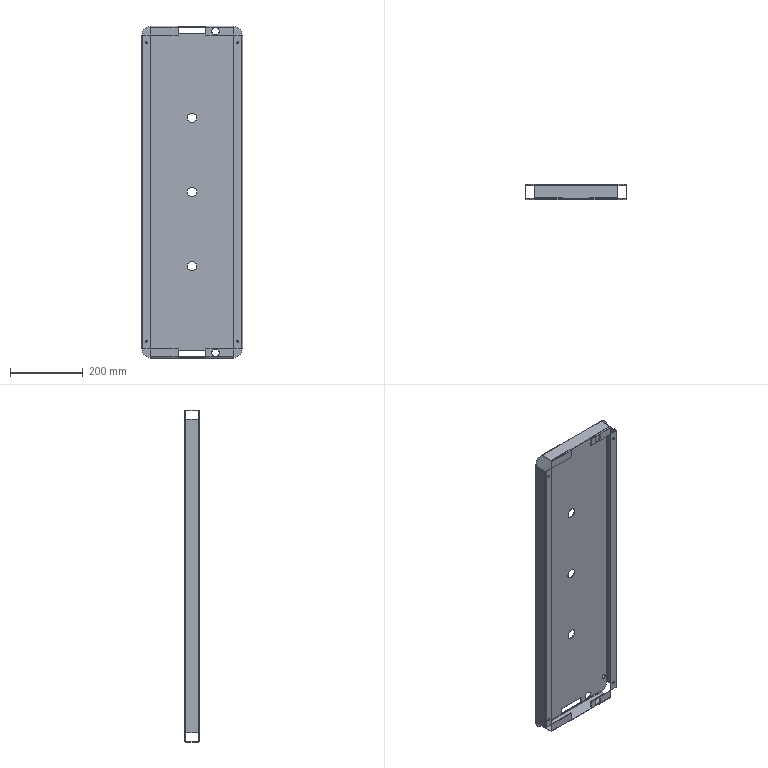Part | NX | features BREP 1 | 1 solid | 164 faces | box 277.825 x 39.827 x 910.285 mm | volume 558823 mm3 | plane 102 | cylinder 62 | commonest cylinder face diameters 3.175 x10 6.172 x10 6.096 x8 12.7 x8 20.32 x8 25.4 x6